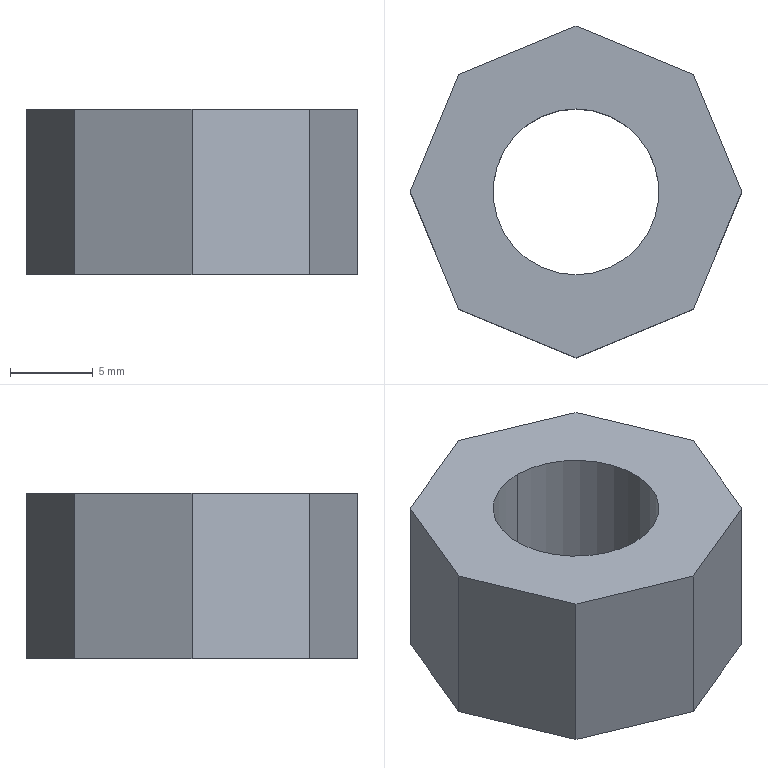Part | SolidWorks | features BaseBody 1 | 1 solid | 12 faces | box 20 x 20 x 10 mm | volume 2043 mm3 | plane 10 | cylinder 2 | commonest cylinder face diameters 10 x2
STEP:
#1=CARTESIAN_POINT('',(358.959,52.138,468.));
#2=VERTEX_POINT('',#1);
#3=CARTESIAN_POINT('',(358.959,62.138,468.));
#4=VERTEX_POINT('',#3);
#5=CARTESIAN_POINT('',(358.959,57.138,468.));
#6=DIRECTION('',(0.,0.,-1.));
#7=DIRECTION('',(0.,1.,0.));
#8=AXIS2_PLACEMENT_3D('',#5,#6,#7);
#9=CIRCLE('',#8,5.);
#10=EDGE_CURVE('',#2,#4,#9,.T.);
#11=ORIENTED_EDGE('',*,*,#10,.T.);
#12=CARTESIAN_POINT('',(358.959,62.138,478.));
#13=VERTEX_POINT('',#12);
#14=CARTESIAN_POINT('',(358.959,62.138,468.));
#15=DIRECTION('',(0.,0.,1.));
#16=VECTOR('',#15,1000.);
#17=LINE('',#14,#16);
#18=EDGE_CURVE('',#4,#13,#17,.T.);
#19=ORIENTED_EDGE('',*,*,#18,.T.);
#20=CARTESIAN_POINT('',(358.959,52.138,478.));
#21=VERTEX_POINT('',#20);
#22=CARTESIAN_POINT('',(358.959,57.138,478.));
#23=DIRECTION('',(0.,0.,-1.));
#24=DIRECTION('',(0.,1.,0.));
#25=AXIS2_PLACEMENT_3D('',#22,#23,#24);
#26=CIRCLE('',#25,5.);
#27=EDGE_CURVE('',#21,#13,#26,.T.);
#28=ORIENTED_EDGE('',*,*,#27,.F.);
#29=CARTESIAN_POINT('',(358.959,52.138,468.));
#30=DIRECTION('',(0.,0.,1.));
#31=VECTOR('',#30,1000.);
#32=LINE('',#29,#31);
#33=EDGE_CURVE('',#2,#21,#32,.T.);
#34=ORIENTED_EDGE('',*,*,#33,.F.);
#35=EDGE_LOOP('',(#11,#19,#28,#34));
#36=FACE_OUTER_BOUND('',#35,.T.);
#37=CARTESIAN_POINT('',(358.959,57.138,468.));
#38=DIRECTION('',(0.,0.,1.));
#39=DIRECTION('',(0.,-1.,0.));
#40=AXIS2_PLACEMENT_3D('',#37,#38,#39);
#41=CYLINDRICAL_SURFACE('',#40,5.);
#42=ADVANCED_FACE('',(#36),#41,.F.);
#43=CARTESIAN_POINT('',(358.959,67.138,468.));
#44=VERTEX_POINT('',#43);
#45=CARTESIAN_POINT('',(366.03,64.209,468.));
#46=VERTEX_POINT('',#45);
#47=CARTESIAN_POINT('',(358.959,67.138,468.));
#48=DIRECTION('',(0.9239,-0.3827,0.));
#49=VECTOR('',#48,1000.);
#50=LINE('',#47,#49);
#51=EDGE_CURVE('',#44,#46,#50,.T.);
#52=ORIENTED_EDGE('',*,*,#51,.T.);
#53=CARTESIAN_POINT('',(368.959,57.138,468.));
#54=VERTEX_POINT('',#53);
#55=CARTESIAN_POINT('',(366.03,64.209,468.));
#56=DIRECTION('',(0.3827,-0.9239,0.));
#57=VECTOR('',#56,1000.);
#58=LINE('',#55,#57);
#59=EDGE_CURVE('',#46,#54,#58,.T.);
#60=ORIENTED_EDGE('',*,*,#59,.T.);
#61=CARTESIAN_POINT('',(366.03,50.067,468.));
#62=VERTEX_POINT('',#61);
#63=CARTESIAN_POINT('',(366.03,50.067,468.));
#64=DIRECTION('',(-0.3827,-0.9239,0.));
#65=VECTOR('',#64,1000.);
#66=LINE('',#63,#65);
#67=EDGE_CURVE('',#54,#62,#66,.T.);
#68=ORIENTED_EDGE('',*,*,#67,.T.);
#69=CARTESIAN_POINT('',(358.959,47.138,468.));
#70=VERTEX_POINT('',#69);
#71=CARTESIAN_POINT('',(358.959,47.138,468.));
#72=DIRECTION('',(-0.9239,-0.3827,0.));
#73=VECTOR('',#72,1000.);
#74=LINE('',#71,#73);
#75=EDGE_CURVE('',#62,#70,#74,.T.);
#76=ORIENTED_EDGE('',*,*,#75,.T.);
#77=CARTESIAN_POINT('',(351.888,50.067,468.));
#78=VERTEX_POINT('',#77);
#79=CARTESIAN_POINT('',(351.888,50.067,468.));
#80=DIRECTION('',(-0.9239,0.3827,0.));
#81=VECTOR('',#80,1000.);
#82=LINE('',#79,#81);
#83=EDGE_CURVE('',#70,#78,#82,.T.);
#84=ORIENTED_EDGE('',*,*,#83,.T.);
#85=CARTESIAN_POINT('',(348.959,57.138,468.));
#86=VERTEX_POINT('',#85);
#87=CARTESIAN_POINT('',(351.888,50.067,468.));
#88=DIRECTION('',(-0.3827,0.9239,0.));
#89=VECTOR('',#88,1000.);
#90=LINE('',#87,#89);
#91=EDGE_CURVE('',#78,#86,#90,.T.);
#92=ORIENTED_EDGE('',*,*,#91,.T.);
#93=CARTESIAN_POINT('',(351.888,64.209,468.));
#94=VERTEX_POINT('',#93);
#95=CARTESIAN_POINT('',(351.888,64.209,468.));
#96=DIRECTION('',(0.3827,0.9239,0.));
#97=VECTOR('',#96,1000.);
#98=LINE('',#95,#97);
#99=EDGE_CURVE('',#86,#94,#98,.T.);
#100=ORIENTED_EDGE('',*,*,#99,.T.);
#101=CARTESIAN_POINT('',(351.888,64.209,468.));
#102=DIRECTION('',(0.9239,0.3827,0.));
#103=VECTOR('',#102,1000.);
#104=LINE('',#101,#103);
#105=EDGE_CURVE('',#94,#44,#104,.T.);
#106=ORIENTED_EDGE('',*,*,#105,.T.);
#107=EDGE_LOOP('',(#52,#60,#68,#76,#84,#92,#100,#106));
#108=FACE_OUTER_BOUND('',#107,.T.);
#109=ORIENTED_EDGE('',*,*,#10,.F.);
#110=CARTESIAN_POINT('',(358.959,57.138,468.));
#111=DIRECTION('',(0.,0.,-1.));
#112=DIRECTION('',(0.,1.,0.));
#113=AXIS2_PLACEMENT_3D('',#110,#111,#112);
#114=CIRCLE('',#113,5.);
#115=EDGE_CURVE('',#4,#2,#114,.T.);
#116=ORIENTED_EDGE('',*,*,#115,.F.);
#117=EDGE_LOOP('',(#109,#116));
#118=FACE_BOUND('',#117,.T.);
#119=CARTESIAN_POINT('',(358.959,57.138,468.));
#120=DIRECTION('',(0.,0.,1.));
#121=DIRECTION('',(0.,-1.,0.));
#122=AXIS2_PLACEMENT_3D('',#119,#120,#121);
#123=PLANE('',#122);
#124=ADVANCED_FACE('',(#108,#118),#123,.F.);
#125=CARTESIAN_POINT('',(358.959,67.138,478.));
#126=VERTEX_POINT('',#125);
#127=CARTESIAN_POINT('',(366.03,64.209,478.));
#128=VERTEX_POINT('',#127);
#129=CARTESIAN_POINT('',(358.959,67.138,478.));
#130=DIRECTION('',(0.9239,-0.3827,0.));
#131=VECTOR('',#130,1000.);
#132=LINE('',#129,#131);
#133=EDGE_CURVE('',#126,#128,#132,.T.);
#134=ORIENTED_EDGE('',*,*,#133,.F.);
#135=CARTESIAN_POINT('',(351.888,64.209,478.));
#136=VERTEX_POINT('',#135);
#137=CARTESIAN_POINT('',(351.888,64.209,478.));
#138=DIRECTION('',(0.9239,0.3827,0.));
#139=VECTOR('',#138,1000.);
#140=LINE('',#137,#139);
#141=EDGE_CURVE('',#136,#126,#140,.T.);
#142=ORIENTED_EDGE('',*,*,#141,.F.);
#143=CARTESIAN_POINT('',(348.959,57.138,478.));
#144=VERTEX_POINT('',#143);
#145=CARTESIAN_POINT('',(351.888,64.209,478.));
#146=DIRECTION('',(0.3827,0.9239,0.));
#147=VECTOR('',#146,1000.);
#148=LINE('',#145,#147);
#149=EDGE_CURVE('',#144,#136,#148,.T.);
#150=ORIENTED_EDGE('',*,*,#149,.F.);
#151=CARTESIAN_POINT('',(351.888,50.067,478.));
#152=VERTEX_POINT('',#151);
#153=CARTESIAN_POINT('',(351.888,50.067,478.));
#154=DIRECTION('',(-0.3827,0.9239,0.));
#155=VECTOR('',#154,1000.);
#156=LINE('',#153,#155);
#157=EDGE_CURVE('',#152,#144,#156,.T.);
#158=ORIENTED_EDGE('',*,*,#157,.F.);
#159=CARTESIAN_POINT('',(358.959,47.138,478.));
#160=VERTEX_POINT('',#159);
#161=CARTESIAN_POINT('',(351.888,50.067,478.));
#162=DIRECTION('',(-0.9239,0.3827,0.));
#163=VECTOR('',#162,1000.);
#164=LINE('',#161,#163);
#165=EDGE_CURVE('',#160,#152,#164,.T.);
#166=ORIENTED_EDGE('',*,*,#165,.F.);
#167=CARTESIAN_POINT('',(366.03,50.067,478.));
#168=VERTEX_POINT('',#167);
#169=CARTESIAN_POINT('',(358.959,47.138,478.));
#170=DIRECTION('',(-0.9239,-0.3827,0.));
#171=VECTOR('',#170,1000.);
#172=LINE('',#169,#171);
#173=EDGE_CURVE('',#168,#160,#172,.T.);
#174=ORIENTED_EDGE('',*,*,#173,.F.);
#175=CARTESIAN_POINT('',(368.959,57.138,478.));
#176=VERTEX_POINT('',#175);
#177=CARTESIAN_POINT('',(366.03,50.067,478.));
#178=DIRECTION('',(-0.3827,-0.9239,0.));
#179=VECTOR('',#178,1000.);
#180=LINE('',#177,#179);
#181=EDGE_CURVE('',#176,#168,#180,.T.);
#182=ORIENTED_EDGE('',*,*,#181,.F.);
#183=CARTESIAN_POINT('',(366.03,64.209,478.));
#184=DIRECTION('',(0.3827,-0.9239,0.));
#185=VECTOR('',#184,1000.);
#186=LINE('',#183,#185);
#187=EDGE_CURVE('',#128,#176,#186,.T.);
#188=ORIENTED_EDGE('',*,*,#187,.F.);
#189=EDGE_LOOP('',(#134,#142,#150,#158,#166,#174,#182,#188));
#190=FACE_OUTER_BOUND('',#189,.T.);
#191=ORIENTED_EDGE('',*,*,#27,.T.);
#192=CARTESIAN_POINT('',(358.959,57.138,478.));
#193=DIRECTION('',(0.,0.,-1.));
#194=DIRECTION('',(0.,1.,0.));
#195=AXIS2_PLACEMENT_3D('',#192,#193,#194);
#196=CIRCLE('',#195,5.);
#197=EDGE_CURVE('',#13,#21,#196,.T.);
#198=ORIENTED_EDGE('',*,*,#197,.T.);
#199=EDGE_LOOP('',(#191,#198));
#200=FACE_BOUND('',#199,.T.);
#201=CARTESIAN_POINT('',(358.959,57.138,478.));
#202=DIRECTION('',(0.,0.,1.));
#203=DIRECTION('',(0.,-1.,0.));
#204=AXIS2_PLACEMENT_3D('',#201,#202,#203);
#205=PLANE('',#204);
#206=ADVANCED_FACE('',(#190,#200),#205,.T.);
#207=ORIENTED_EDGE('',*,*,#133,.T.);
#208=CARTESIAN_POINT('',(366.03,64.209,468.));
#209=DIRECTION('',(0.,0.,1.));
#210=VECTOR('',#209,1000.);
#211=LINE('',#208,#210);
#212=EDGE_CURVE('',#46,#128,#211,.T.);
#213=ORIENTED_EDGE('',*,*,#212,.F.);
#214=ORIENTED_EDGE('',*,*,#51,.F.);
#215=CARTESIAN_POINT('',(358.959,67.138,468.));
#216=DIRECTION('',(0.,0.,1.));
#217=VECTOR('',#216,1000.);
#218=LINE('',#215,#217);
#219=EDGE_CURVE('',#44,#126,#218,.T.);
#220=ORIENTED_EDGE('',*,*,#219,.T.);
#221=EDGE_LOOP('',(#207,#213,#214,#220));
#222=FACE_OUTER_BOUND('',#221,.T.);
#223=CARTESIAN_POINT('',(358.959,67.138,468.));
#224=DIRECTION('',(-0.3827,-0.9239,0.));
#225=DIRECTION('',(-0.9239,0.3827,0.));
#226=AXIS2_PLACEMENT_3D('',#223,#224,#225);
#227=PLANE('',#226);
#228=ADVANCED_FACE('',(#222),#227,.F.);
#229=ORIENTED_EDGE('',*,*,#187,.T.);
#230=CARTESIAN_POINT('',(368.959,57.138,468.));
#231=DIRECTION('',(0.,0.,1.));
#232=VECTOR('',#231,1000.);
#233=LINE('',#230,#232);
#234=EDGE_CURVE('',#54,#176,#233,.T.);
#235=ORIENTED_EDGE('',*,*,#234,.F.);
#236=ORIENTED_EDGE('',*,*,#59,.F.);
#237=ORIENTED_EDGE('',*,*,#212,.T.);
#238=EDGE_LOOP('',(#229,#235,#236,#237));
#239=FACE_OUTER_BOUND('',#238,.T.);
#240=CARTESIAN_POINT('',(366.03,64.209,468.));
#241=DIRECTION('',(-0.9239,-0.3827,0.));
#242=DIRECTION('',(-0.3827,0.9239,0.));
#243=AXIS2_PLACEMENT_3D('',#240,#241,#242);
#244=PLANE('',#243);
#245=ADVANCED_FACE('',(#239),#244,.F.);
#246=ORIENTED_EDGE('',*,*,#181,.T.);
#247=CARTESIAN_POINT('',(366.03,50.067,468.));
#248=DIRECTION('',(0.,0.,1.));
#249=VECTOR('',#248,1000.);
#250=LINE('',#247,#249);
#251=EDGE_CURVE('',#62,#168,#250,.T.);
#252=ORIENTED_EDGE('',*,*,#251,.F.);
#253=ORIENTED_EDGE('',*,*,#67,.F.);
#254=ORIENTED_EDGE('',*,*,#234,.T.);
#255=EDGE_LOOP('',(#246,#252,#253,#254));
#256=FACE_OUTER_BOUND('',#255,.T.);
#257=CARTESIAN_POINT('',(366.03,50.067,468.));
#258=DIRECTION('',(-0.9239,0.3827,0.));
#259=DIRECTION('',(0.3827,0.9239,0.));
#260=AXIS2_PLACEMENT_3D('',#257,#258,#259);
#261=PLANE('',#260);
#262=ADVANCED_FACE('',(#256),#261,.F.);
#263=ORIENTED_EDGE('',*,*,#173,.T.);
#264=CARTESIAN_POINT('',(358.959,47.138,468.));
#265=DIRECTION('',(0.,0.,1.));
#266=VECTOR('',#265,1000.);
#267=LINE('',#264,#266);
#268=EDGE_CURVE('',#70,#160,#267,.T.);
#269=ORIENTED_EDGE('',*,*,#268,.F.);
#270=ORIENTED_EDGE('',*,*,#75,.F.);
#271=ORIENTED_EDGE('',*,*,#251,.T.);
#272=EDGE_LOOP('',(#263,#269,#270,#271));
#273=FACE_OUTER_BOUND('',#272,.T.);
#274=CARTESIAN_POINT('',(358.959,47.138,468.));
#275=DIRECTION('',(-0.3827,0.9239,0.));
#276=DIRECTION('',(0.9239,0.3827,0.));
#277=AXIS2_PLACEMENT_3D('',#274,#275,#276);
#278=PLANE('',#277);
#279=ADVANCED_FACE('',(#273),#278,.F.);
#280=ORIENTED_EDGE('',*,*,#165,.T.);
#281=CARTESIAN_POINT('',(351.888,50.067,468.));
#282=DIRECTION('',(0.,0.,1.));
#283=VECTOR('',#282,1000.);
#284=LINE('',#281,#283);
#285=EDGE_CURVE('',#78,#152,#284,.T.);
#286=ORIENTED_EDGE('',*,*,#285,.F.);
#287=ORIENTED_EDGE('',*,*,#83,.F.);
#288=ORIENTED_EDGE('',*,*,#268,.T.);
#289=EDGE_LOOP('',(#280,#286,#287,#288));
#290=FACE_OUTER_BOUND('',#289,.T.);
#291=CARTESIAN_POINT('',(351.888,50.067,468.));
#292=DIRECTION('',(0.3827,0.9239,0.));
#293=DIRECTION('',(0.9239,-0.3827,0.));
#294=AXIS2_PLACEMENT_3D('',#291,#292,#293);
#295=PLANE('',#294);
#296=ADVANCED_FACE('',(#290),#295,.F.);
#297=ORIENTED_EDGE('',*,*,#157,.T.);
#298=CARTESIAN_POINT('',(348.959,57.138,468.));
#299=DIRECTION('',(0.,0.,1.));
#300=VECTOR('',#299,1000.);
#301=LINE('',#298,#300);
#302=EDGE_CURVE('',#86,#144,#301,.T.);
#303=ORIENTED_EDGE('',*,*,#302,.F.);
#304=ORIENTED_EDGE('',*,*,#91,.F.);
#305=ORIENTED_EDGE('',*,*,#285,.T.);
#306=EDGE_LOOP('',(#297,#303,#304,#305));
#307=FACE_OUTER_BOUND('',#306,.T.);
#308=CARTESIAN_POINT('',(351.888,50.067,468.));
#309=DIRECTION('',(0.9239,0.3827,0.));
#310=DIRECTION('',(0.3827,-0.9239,0.));
#311=AXIS2_PLACEMENT_3D('',#308,#309,#310);
#312=PLANE('',#311);
#313=ADVANCED_FACE('',(#307),#312,.F.);
#314=ORIENTED_EDGE('',*,*,#149,.T.);
#315=CARTESIAN_POINT('',(351.888,64.209,468.));
#316=DIRECTION('',(0.,0.,1.));
#317=VECTOR('',#316,1000.);
#318=LINE('',#315,#317);
#319=EDGE_CURVE('',#94,#136,#318,.T.);
#320=ORIENTED_EDGE('',*,*,#319,.F.);
#321=ORIENTED_EDGE('',*,*,#99,.F.);
#322=ORIENTED_EDGE('',*,*,#302,.T.);
#323=EDGE_LOOP('',(#314,#320,#321,#322));
#324=FACE_OUTER_BOUND('',#323,.T.);
#325=CARTESIAN_POINT('',(351.888,64.209,468.));
#326=DIRECTION('',(0.9239,-0.3827,0.));
#327=DIRECTION('',(-0.3827,-0.9239,0.));
#328=AXIS2_PLACEMENT_3D('',#325,#326,#327);
#329=PLANE('',#328);
#330=ADVANCED_FACE('',(#324),#329,.F.);
#331=ORIENTED_EDGE('',*,*,#141,.T.);
#332=ORIENTED_EDGE('',*,*,#219,.F.);
#333=ORIENTED_EDGE('',*,*,#105,.F.);
#334=ORIENTED_EDGE('',*,*,#319,.T.);
#335=EDGE_LOOP('',(#331,#332,#333,#334));
#336=FACE_OUTER_BOUND('',#335,.T.);
#337=CARTESIAN_POINT('',(351.888,64.209,468.));
#338=DIRECTION('',(0.3827,-0.9239,0.));
#339=DIRECTION('',(-0.9239,-0.3827,0.));
#340=AXIS2_PLACEMENT_3D('',#337,#338,#339);
#341=PLANE('',#340);
#342=ADVANCED_FACE('',(#336),#341,.F.);
#343=ORIENTED_EDGE('',*,*,#18,.F.);
#344=ORIENTED_EDGE('',*,*,#115,.T.);
#345=ORIENTED_EDGE('',*,*,#33,.T.);
#346=ORIENTED_EDGE('',*,*,#197,.F.);
#347=EDGE_LOOP('',(#343,#344,#345,#346));
#348=FACE_OUTER_BOUND('',#347,.T.);
#349=CARTESIAN_POINT('',(358.959,57.138,468.));
#350=DIRECTION('',(0.,0.,1.));
#351=DIRECTION('',(0.,-1.,0.));
#352=AXIS2_PLACEMENT_3D('',#349,#350,#351);
#353=CYLINDRICAL_SURFACE('',#352,5.);
#354=ADVANCED_FACE('',(#348),#353,.F.);
#355=CLOSED_SHELL('',(#42,#124,#206,#228,#245,#262,#279,#296,#313,#330,#342,#354));
#356=MANIFOLD_SOLID_BREP('',#355);
#357=CARTESIAN_POINT('',(0.,0.,0.));
#358=DIRECTION('',(0.,0.,1.));
#359=DIRECTION('',(1.,0.,0.));
#360=AXIS2_PLACEMENT_3D('',#357,#358,#359);
#361=(LENGTH_UNIT()NAMED_UNIT(*)SI_UNIT(.MILLI.,.METRE.));
#362=UNCERTAINTY_MEASURE_WITH_UNIT(LENGTH_MEASURE(0.00001),#361,'','');
#363=(NAMED_UNIT(*)PLANE_ANGLE_UNIT()SI_UNIT($,.RADIAN.));
#364=(NAMED_UNIT(*)SI_UNIT($,.STERADIAN.)SOLID_ANGLE_UNIT());
#365=(GEOMETRIC_REPRESENTATION_CONTEXT(3)GLOBAL_UNCERTAINTY_ASSIGNED_CONTEXT((#362))GLOBAL_UNIT_ASSIGNED_CONTEXT((#361,#363,#364))REPRESENTATION_CONTEXT('',''));
#366=ADVANCED_BREP_SHAPE_REPRESENTATION('',(#356,#360),#365);